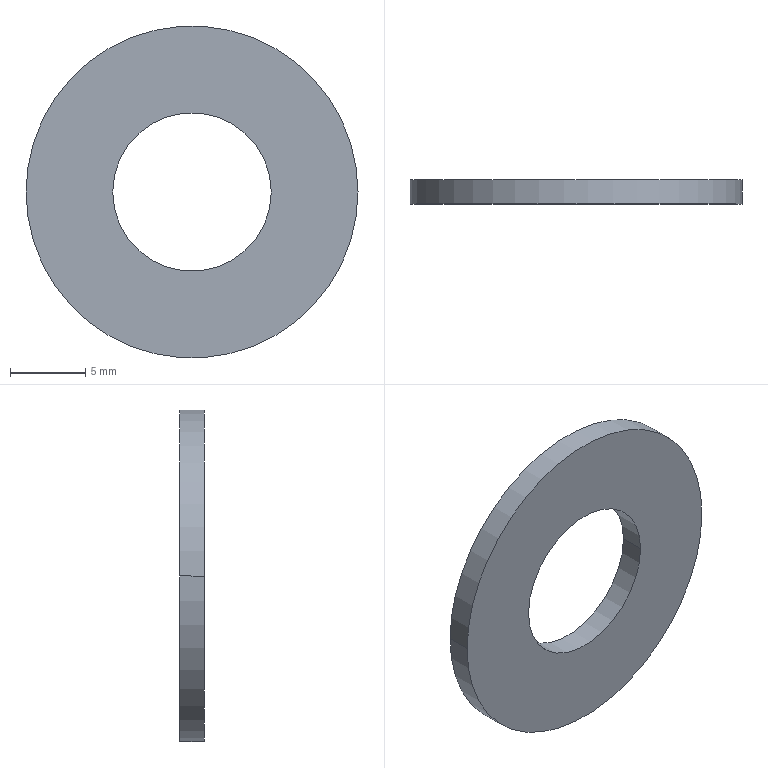Part | STEP file | ZZ21-M10 | 1 solid | 6 faces | box 22 x 1.6 x 22 mm | volume 469.668 mm3 | cylinder 4 | plane 2 | commonest cylinder face diameters 10.5 x2 22 x2
STEP:
#1=CARTESIAN_POINT('',(0.,0.,0.));
#2=DIRECTION('',(0.,0.,1.));
#3=DIRECTION('',(1.,0.,0.));
#4=AXIS2_PLACEMENT_3D('',#1,#2,#3);
#5=CARTESIAN_POINT('',(-5.25,0.,0.));
#6=VERTEX_POINT('',#5);
#7=CARTESIAN_POINT('',(-5.25,1.6,0.));
#8=VERTEX_POINT('',#7);
#9=CARTESIAN_POINT('',(-5.25,0.,0.));
#10=DIRECTION('',(0.,1.,0.));
#11=VECTOR('',#10,1.);
#12=LINE('',#9,#11);
#13=CARTESIAN_POINT('',(0.,0.,0.));
#14=DIRECTION('',(0.,1.,0.));
#15=DIRECTION('',(-1.,0.,0.));
#16=AXIS2_PLACEMENT_3D('',#13,#14,#15);
#17=CYLINDRICAL_SURFACE('',#16,5.25);
#18=CARTESIAN_POINT('',(6.283,0.));
#19=DIRECTION('',(0.,1.));
#20=VECTOR('',#19,1.);
#21=LINE('',#18,#20);
#22=(GEOMETRIC_REPRESENTATION_CONTEXT(2)PARAMETRIC_REPRESENTATION_CONTEXT()REPRESENTATION_CONTEXT('',''));
#23=DEFINITIONAL_REPRESENTATION('',(#21),#22);
#24=PCURVE('',#17,#23);
#25=CARTESIAN_POINT('',(0.,0.,0.));
#26=DIRECTION('',(0.,1.,0.));
#27=DIRECTION('',(-1.,0.,0.));
#28=AXIS2_PLACEMENT_3D('',#25,#26,#27);
#29=CYLINDRICAL_SURFACE('',#28,5.25);
#30=CARTESIAN_POINT('',(0.,0.));
#31=DIRECTION('',(0.,1.));
#32=VECTOR('',#31,1.);
#33=LINE('',#30,#32);
#34=(GEOMETRIC_REPRESENTATION_CONTEXT(2)PARAMETRIC_REPRESENTATION_CONTEXT()REPRESENTATION_CONTEXT('',''));
#35=DEFINITIONAL_REPRESENTATION('',(#33),#34);
#36=PCURVE('',#29,#35);
#37=SURFACE_CURVE('',#12,(#24,#36),.PCURVE_S1.);
#38=EDGE_CURVE('',#6,#8,#37,.T.);
#39=ORIENTED_EDGE('',*,*,#38,.T.);
#40=CARTESIAN_POINT('',(5.25,1.6,0.));
#41=VERTEX_POINT('',#40);
#42=CARTESIAN_POINT('',(0.,1.6,0.));
#43=DIRECTION('',(0.,-1.,0.));
#44=DIRECTION('',(1.,0.,0.));
#45=AXIS2_PLACEMENT_3D('',#42,#43,#44);
#46=CIRCLE('',#45,5.25);
#47=CARTESIAN_POINT('',(9.425,1.6));
#48=DIRECTION('',(-1.,0.));
#49=VECTOR('',#48,1.);
#50=LINE('',#47,#49);
#51=(GEOMETRIC_REPRESENTATION_CONTEXT(2)PARAMETRIC_REPRESENTATION_CONTEXT()REPRESENTATION_CONTEXT('',''));
#52=DEFINITIONAL_REPRESENTATION('',(#50),#51);
#53=PCURVE('',#17,#52);
#54=CARTESIAN_POINT('',(0.,1.6,0.));
#55=DIRECTION('',(0.,1.,0.));
#56=DIRECTION('',(-1.,0.,0.));
#57=AXIS2_PLACEMENT_3D('',#54,#55,#56);
#58=PLANE('',#57);
#59=CARTESIAN_POINT('',(-5.25,0.));
#60=CARTESIAN_POINT('',(-5.25,9.093));
#61=CARTESIAN_POINT('',(2.625,4.547));
#62=CARTESIAN_POINT('',(10.5,0.));
#63=CARTESIAN_POINT('',(2.625,-4.547));
#64=CARTESIAN_POINT('',(-5.25,-9.093));
#65=CARTESIAN_POINT('',(-5.25,0.));
#66=(BOUNDED_CURVE()B_SPLINE_CURVE(2,(#59,#60,#61,#62,#63,#64,#65),.UNSPECIFIED.,.T.,.F.)B_SPLINE_CURVE_WITH_KNOTS((1,2,2,2,2,1),(-2.094,0.,2.094,4.189,6.283,8.378),.UNSPECIFIED.)CURVE()GEOMETRIC_REPRESENTATION_ITEM()RATIONAL_B_SPLINE_CURVE((1.,0.5,1.,0.5,1.,0.5,1.))REPRESENTATION_ITEM(''));
#67=(GEOMETRIC_REPRESENTATION_CONTEXT(2)PARAMETRIC_REPRESENTATION_CONTEXT()REPRESENTATION_CONTEXT('',''));
#68=DEFINITIONAL_REPRESENTATION('',(#66),#67);
#69=PCURVE('',#58,#68);
#70=SURFACE_CURVE('',#46,(#53,#69),.PCURVE_S1.);
#71=EDGE_CURVE('',#8,#41,#70,.T.);
#72=ORIENTED_EDGE('',*,*,#71,.T.);
#73=CARTESIAN_POINT('',(5.25,0.,0.));
#74=VERTEX_POINT('',#73);
#75=CARTESIAN_POINT('',(5.25,0.,0.));
#76=DIRECTION('',(0.,1.,0.));
#77=VECTOR('',#76,1.);
#78=LINE('',#75,#77);
#79=CARTESIAN_POINT('',(3.142,0.));
#80=DIRECTION('',(0.,1.));
#81=VECTOR('',#80,1.);
#82=LINE('',#79,#81);
#83=(GEOMETRIC_REPRESENTATION_CONTEXT(2)PARAMETRIC_REPRESENTATION_CONTEXT()REPRESENTATION_CONTEXT('',''));
#84=DEFINITIONAL_REPRESENTATION('',(#82),#83);
#85=PCURVE('',#17,#84);
#86=CARTESIAN_POINT('',(3.142,0.));
#87=DIRECTION('',(0.,1.));
#88=VECTOR('',#87,1.);
#89=LINE('',#86,#88);
#90=(GEOMETRIC_REPRESENTATION_CONTEXT(2)PARAMETRIC_REPRESENTATION_CONTEXT()REPRESENTATION_CONTEXT('',''));
#91=DEFINITIONAL_REPRESENTATION('',(#89),#90);
#92=PCURVE('',#29,#91);
#93=SURFACE_CURVE('',#78,(#85,#92),.PCURVE_S1.);
#94=EDGE_CURVE('',#74,#41,#93,.T.);
#95=ORIENTED_EDGE('',*,*,#94,.F.);
#96=CARTESIAN_POINT('',(0.,0.,0.));
#97=DIRECTION('',(0.,1.,0.));
#98=DIRECTION('',(-1.,0.,0.));
#99=AXIS2_PLACEMENT_3D('',#96,#97,#98);
#100=CIRCLE('',#99,5.25);
#101=CARTESIAN_POINT('',(0.,0.));
#102=DIRECTION('',(1.,0.));
#103=VECTOR('',#102,1.);
#104=LINE('',#101,#103);
#105=(GEOMETRIC_REPRESENTATION_CONTEXT(2)PARAMETRIC_REPRESENTATION_CONTEXT()REPRESENTATION_CONTEXT('',''));
#106=DEFINITIONAL_REPRESENTATION('',(#104),#105);
#107=PCURVE('',#17,#106);
#108=CARTESIAN_POINT('',(0.,0.,0.));
#109=DIRECTION('',(0.,-1.,0.));
#110=DIRECTION('',(1.,0.,0.));
#111=AXIS2_PLACEMENT_3D('',#108,#109,#110);
#112=PLANE('',#111);
#113=CARTESIAN_POINT('',(-5.25,0.));
#114=CARTESIAN_POINT('',(-5.25,9.093));
#115=CARTESIAN_POINT('',(2.625,4.547));
#116=CARTESIAN_POINT('',(10.5,0.));
#117=CARTESIAN_POINT('',(2.625,-4.547));
#118=CARTESIAN_POINT('',(-5.25,-9.093));
#119=CARTESIAN_POINT('',(-5.25,0.));
#120=(BOUNDED_CURVE()B_SPLINE_CURVE(2,(#113,#114,#115,#116,#117,#118,#119),.UNSPECIFIED.,.T.,.F.)B_SPLINE_CURVE_WITH_KNOTS((1,2,2,2,2,1),(-2.094,0.,2.094,4.189,6.283,8.378),.UNSPECIFIED.)CURVE()GEOMETRIC_REPRESENTATION_ITEM()RATIONAL_B_SPLINE_CURVE((1.,0.5,1.,0.5,1.,0.5,1.))REPRESENTATION_ITEM(''));
#121=(GEOMETRIC_REPRESENTATION_CONTEXT(2)PARAMETRIC_REPRESENTATION_CONTEXT()REPRESENTATION_CONTEXT('',''));
#122=DEFINITIONAL_REPRESENTATION('',(#120),#121);
#123=PCURVE('',#112,#122);
#124=SURFACE_CURVE('',#100,(#107,#123),.PCURVE_S1.);
#125=EDGE_CURVE('',#74,#6,#124,.T.);
#126=ORIENTED_EDGE('',*,*,#125,.T.);
#127=EDGE_LOOP('',(#39,#72,#95,#126));
#128=FACE_BOUND('',#127,.F.);
#129=ADVANCED_FACE('',(#128),#17,.F.);
#130=CARTESIAN_POINT('',(-11.,0.,0.));
#131=VERTEX_POINT('',#130);
#132=CARTESIAN_POINT('',(11.,0.,0.));
#133=VERTEX_POINT('',#132);
#134=CARTESIAN_POINT('',(0.,0.,0.));
#135=DIRECTION('',(0.,1.,0.));
#136=DIRECTION('',(-1.,0.,0.));
#137=AXIS2_PLACEMENT_3D('',#134,#135,#136);
#138=CIRCLE('',#137,11.);
#139=CARTESIAN_POINT('',(0.,0.,0.));
#140=DIRECTION('',(0.,1.,0.));
#141=DIRECTION('',(-1.,0.,0.));
#142=AXIS2_PLACEMENT_3D('',#139,#140,#141);
#143=CYLINDRICAL_SURFACE('',#142,11.);
#144=CARTESIAN_POINT('',(0.,0.));
#145=DIRECTION('',(1.,0.));
#146=VECTOR('',#145,1.);
#147=LINE('',#144,#146);
#148=(GEOMETRIC_REPRESENTATION_CONTEXT(2)PARAMETRIC_REPRESENTATION_CONTEXT()REPRESENTATION_CONTEXT('',''));
#149=DEFINITIONAL_REPRESENTATION('',(#147),#148);
#150=PCURVE('',#143,#149);
#151=CARTESIAN_POINT('',(-11.,0.));
#152=CARTESIAN_POINT('',(-11.,19.053));
#153=CARTESIAN_POINT('',(5.5,9.526));
#154=CARTESIAN_POINT('',(22.,0.));
#155=CARTESIAN_POINT('',(5.5,-9.526));
#156=CARTESIAN_POINT('',(-11.,-19.053));
#157=CARTESIAN_POINT('',(-11.,0.));
#158=(BOUNDED_CURVE()B_SPLINE_CURVE(2,(#151,#152,#153,#154,#155,#156,#157),.UNSPECIFIED.,.T.,.F.)B_SPLINE_CURVE_WITH_KNOTS((1,2,2,2,2,1),(-2.094,0.,2.094,4.189,6.283,8.378),.UNSPECIFIED.)CURVE()GEOMETRIC_REPRESENTATION_ITEM()RATIONAL_B_SPLINE_CURVE((1.,0.5,1.,0.5,1.,0.5,1.))REPRESENTATION_ITEM(''));
#159=(GEOMETRIC_REPRESENTATION_CONTEXT(2)PARAMETRIC_REPRESENTATION_CONTEXT()REPRESENTATION_CONTEXT('',''));
#160=DEFINITIONAL_REPRESENTATION('',(#158),#159);
#161=PCURVE('',#112,#160);
#162=SURFACE_CURVE('',#138,(#150,#161),.PCURVE_S1.);
#163=EDGE_CURVE('',#131,#133,#162,.T.);
#164=ORIENTED_EDGE('',*,*,#163,.T.);
#165=CARTESIAN_POINT('',(11.,1.6,0.));
#166=VERTEX_POINT('',#165);
#167=CARTESIAN_POINT('',(11.,0.,0.));
#168=DIRECTION('',(0.,1.,0.));
#169=VECTOR('',#168,1.);
#170=LINE('',#167,#169);
#171=CARTESIAN_POINT('',(3.142,0.));
#172=DIRECTION('',(0.,1.));
#173=VECTOR('',#172,1.);
#174=LINE('',#171,#173);
#175=(GEOMETRIC_REPRESENTATION_CONTEXT(2)PARAMETRIC_REPRESENTATION_CONTEXT()REPRESENTATION_CONTEXT('',''));
#176=DEFINITIONAL_REPRESENTATION('',(#174),#175);
#177=PCURVE('',#143,#176);
#178=CARTESIAN_POINT('',(0.,0.,0.));
#179=DIRECTION('',(0.,1.,0.));
#180=DIRECTION('',(-1.,0.,0.));
#181=AXIS2_PLACEMENT_3D('',#178,#179,#180);
#182=CYLINDRICAL_SURFACE('',#181,11.);
#183=CARTESIAN_POINT('',(3.142,0.));
#184=DIRECTION('',(0.,1.));
#185=VECTOR('',#184,1.);
#186=LINE('',#183,#185);
#187=(GEOMETRIC_REPRESENTATION_CONTEXT(2)PARAMETRIC_REPRESENTATION_CONTEXT()REPRESENTATION_CONTEXT('',''));
#188=DEFINITIONAL_REPRESENTATION('',(#186),#187);
#189=PCURVE('',#182,#188);
#190=SURFACE_CURVE('',#170,(#177,#189),.PCURVE_S1.);
#191=EDGE_CURVE('',#133,#166,#190,.T.);
#192=ORIENTED_EDGE('',*,*,#191,.T.);
#193=CARTESIAN_POINT('',(-11.,1.6,0.));
#194=VERTEX_POINT('',#193);
#195=CARTESIAN_POINT('',(0.,1.6,0.));
#196=DIRECTION('',(0.,-1.,0.));
#197=DIRECTION('',(1.,0.,0.));
#198=AXIS2_PLACEMENT_3D('',#195,#196,#197);
#199=CIRCLE('',#198,11.);
#200=CARTESIAN_POINT('',(3.142,1.6));
#201=DIRECTION('',(-1.,0.));
#202=VECTOR('',#201,1.);
#203=LINE('',#200,#202);
#204=(GEOMETRIC_REPRESENTATION_CONTEXT(2)PARAMETRIC_REPRESENTATION_CONTEXT()REPRESENTATION_CONTEXT('',''));
#205=DEFINITIONAL_REPRESENTATION('',(#203),#204);
#206=PCURVE('',#143,#205);
#207=CARTESIAN_POINT('',(-11.,0.));
#208=CARTESIAN_POINT('',(-11.,19.053));
#209=CARTESIAN_POINT('',(5.5,9.526));
#210=CARTESIAN_POINT('',(22.,0.));
#211=CARTESIAN_POINT('',(5.5,-9.526));
#212=CARTESIAN_POINT('',(-11.,-19.053));
#213=CARTESIAN_POINT('',(-11.,0.));
#214=(BOUNDED_CURVE()B_SPLINE_CURVE(2,(#207,#208,#209,#210,#211,#212,#213),.UNSPECIFIED.,.T.,.F.)B_SPLINE_CURVE_WITH_KNOTS((1,2,2,2,2,1),(-2.094,0.,2.094,4.189,6.283,8.378),.UNSPECIFIED.)CURVE()GEOMETRIC_REPRESENTATION_ITEM()RATIONAL_B_SPLINE_CURVE((1.,0.5,1.,0.5,1.,0.5,1.))REPRESENTATION_ITEM(''));
#215=(GEOMETRIC_REPRESENTATION_CONTEXT(2)PARAMETRIC_REPRESENTATION_CONTEXT()REPRESENTATION_CONTEXT('',''));
#216=DEFINITIONAL_REPRESENTATION('',(#214),#215);
#217=PCURVE('',#58,#216);
#218=SURFACE_CURVE('',#199,(#206,#217),.PCURVE_S1.);
#219=EDGE_CURVE('',#166,#194,#218,.T.);
#220=ORIENTED_EDGE('',*,*,#219,.T.);
#221=CARTESIAN_POINT('',(-11.,0.,0.));
#222=DIRECTION('',(0.,1.,0.));
#223=VECTOR('',#222,1.);
#224=LINE('',#221,#223);
#225=CARTESIAN_POINT('',(0.,0.));
#226=DIRECTION('',(0.,1.));
#227=VECTOR('',#226,1.);
#228=LINE('',#225,#227);
#229=(GEOMETRIC_REPRESENTATION_CONTEXT(2)PARAMETRIC_REPRESENTATION_CONTEXT()REPRESENTATION_CONTEXT('',''));
#230=DEFINITIONAL_REPRESENTATION('',(#228),#229);
#231=PCURVE('',#143,#230);
#232=CARTESIAN_POINT('',(6.283,0.));
#233=DIRECTION('',(0.,1.));
#234=VECTOR('',#233,1.);
#235=LINE('',#232,#234);
#236=(GEOMETRIC_REPRESENTATION_CONTEXT(2)PARAMETRIC_REPRESENTATION_CONTEXT()REPRESENTATION_CONTEXT('',''));
#237=DEFINITIONAL_REPRESENTATION('',(#235),#236);
#238=PCURVE('',#182,#237);
#239=SURFACE_CURVE('',#224,(#231,#238),.PCURVE_S1.);
#240=EDGE_CURVE('',#131,#194,#239,.T.);
#241=ORIENTED_EDGE('',*,*,#240,.F.);
#242=EDGE_LOOP('',(#164,#192,#220,#241));
#243=FACE_BOUND('',#242,.T.);
#244=ADVANCED_FACE('',(#243),#143,.T.);
#245=ORIENTED_EDGE('',*,*,#71,.T.);
#246=CARTESIAN_POINT('',(0.,1.6,0.));
#247=DIRECTION('',(0.,-1.,0.));
#248=DIRECTION('',(1.,0.,0.));
#249=AXIS2_PLACEMENT_3D('',#246,#247,#248);
#250=CIRCLE('',#249,5.25);
#251=CARTESIAN_POINT('',(-5.25,0.));
#252=CARTESIAN_POINT('',(-5.25,9.093));
#253=CARTESIAN_POINT('',(2.625,4.547));
#254=CARTESIAN_POINT('',(10.5,0.));
#255=CARTESIAN_POINT('',(2.625,-4.547));
#256=CARTESIAN_POINT('',(-5.25,-9.093));
#257=CARTESIAN_POINT('',(-5.25,0.));
#258=(BOUNDED_CURVE()B_SPLINE_CURVE(2,(#251,#252,#253,#254,#255,#256,#257),.UNSPECIFIED.,.T.,.F.)B_SPLINE_CURVE_WITH_KNOTS((1,2,2,2,2,1),(-2.094,0.,2.094,4.189,6.283,8.378),.UNSPECIFIED.)CURVE()GEOMETRIC_REPRESENTATION_ITEM()RATIONAL_B_SPLINE_CURVE((1.,0.5,1.,0.5,1.,0.5,1.))REPRESENTATION_ITEM(''));
#259=(GEOMETRIC_REPRESENTATION_CONTEXT(2)PARAMETRIC_REPRESENTATION_CONTEXT()REPRESENTATION_CONTEXT('',''));
#260=DEFINITIONAL_REPRESENTATION('',(#258),#259);
#261=PCURVE('',#58,#260);
#262=CARTESIAN_POINT('',(3.142,1.6));
#263=DIRECTION('',(-1.,0.));
#264=VECTOR('',#263,1.);
#265=LINE('',#262,#264);
#266=(GEOMETRIC_REPRESENTATION_CONTEXT(2)PARAMETRIC_REPRESENTATION_CONTEXT()REPRESENTATION_CONTEXT('',''));
#267=DEFINITIONAL_REPRESENTATION('',(#265),#266);
#268=PCURVE('',#29,#267);
#269=SURFACE_CURVE('',#250,(#261,#268),.PCURVE_S1.);
#270=EDGE_CURVE('',#41,#8,#269,.T.);
#271=ORIENTED_EDGE('',*,*,#270,.T.);
#272=EDGE_LOOP('',(#245,#271));
#273=FACE_BOUND('',#272,.T.);
#274=CARTESIAN_POINT('',(0.,1.6,0.));
#275=DIRECTION('',(0.,-1.,0.));
#276=DIRECTION('',(1.,0.,0.));
#277=AXIS2_PLACEMENT_3D('',#274,#275,#276);
#278=CIRCLE('',#277,11.);
#279=CARTESIAN_POINT('',(-11.,0.));
#280=CARTESIAN_POINT('',(-11.,19.053));
#281=CARTESIAN_POINT('',(5.5,9.526));
#282=CARTESIAN_POINT('',(22.,0.));
#283=CARTESIAN_POINT('',(5.5,-9.526));
#284=CARTESIAN_POINT('',(-11.,-19.053));
#285=CARTESIAN_POINT('',(-11.,0.));
#286=(BOUNDED_CURVE()B_SPLINE_CURVE(2,(#279,#280,#281,#282,#283,#284,#285),.UNSPECIFIED.,.T.,.F.)B_SPLINE_CURVE_WITH_KNOTS((1,2,2,2,2,1),(-2.094,0.,2.094,4.189,6.283,8.378),.UNSPECIFIED.)CURVE()GEOMETRIC_REPRESENTATION_ITEM()RATIONAL_B_SPLINE_CURVE((1.,0.5,1.,0.5,1.,0.5,1.))REPRESENTATION_ITEM(''));
#287=(GEOMETRIC_REPRESENTATION_CONTEXT(2)PARAMETRIC_REPRESENTATION_CONTEXT()REPRESENTATION_CONTEXT('',''));
#288=DEFINITIONAL_REPRESENTATION('',(#286),#287);
#289=PCURVE('',#58,#288);
#290=CARTESIAN_POINT('',(9.425,1.6));
#291=DIRECTION('',(-1.,0.));
#292=VECTOR('',#291,1.);
#293=LINE('',#290,#292);
#294=(GEOMETRIC_REPRESENTATION_CONTEXT(2)PARAMETRIC_REPRESENTATION_CONTEXT()REPRESENTATION_CONTEXT('',''));
#295=DEFINITIONAL_REPRESENTATION('',(#293),#294);
#296=PCURVE('',#182,#295);
#297=SURFACE_CURVE('',#278,(#289,#296),.PCURVE_S1.);
#298=EDGE_CURVE('',#194,#166,#297,.T.);
#299=ORIENTED_EDGE('',*,*,#298,.F.);
#300=ORIENTED_EDGE('',*,*,#219,.F.);
#301=EDGE_LOOP('',(#299,#300));
#302=FACE_BOUND('',#301,.T.);
#303=ADVANCED_FACE('',(#273,#302),#58,.T.);
#304=CARTESIAN_POINT('',(0.,0.,0.));
#305=DIRECTION('',(0.,1.,0.));
#306=DIRECTION('',(-1.,0.,0.));
#307=AXIS2_PLACEMENT_3D('',#304,#305,#306);
#308=CIRCLE('',#307,5.25);
#309=CARTESIAN_POINT('',(-5.25,0.));
#310=CARTESIAN_POINT('',(-5.25,9.093));
#311=CARTESIAN_POINT('',(2.625,4.547));
#312=CARTESIAN_POINT('',(10.5,0.));
#313=CARTESIAN_POINT('',(2.625,-4.547));
#314=CARTESIAN_POINT('',(-5.25,-9.093));
#315=CARTESIAN_POINT('',(-5.25,0.));
#316=(BOUNDED_CURVE()B_SPLINE_CURVE(2,(#309,#310,#311,#312,#313,#314,#315),.UNSPECIFIED.,.T.,.F.)B_SPLINE_CURVE_WITH_KNOTS((1,2,2,2,2,1),(-2.094,0.,2.094,4.189,6.283,8.378),.UNSPECIFIED.)CURVE()GEOMETRIC_REPRESENTATION_ITEM()RATIONAL_B_SPLINE_CURVE((1.,0.5,1.,0.5,1.,0.5,1.))REPRESENTATION_ITEM(''));
#317=(GEOMETRIC_REPRESENTATION_CONTEXT(2)PARAMETRIC_REPRESENTATION_CONTEXT()REPRESENTATION_CONTEXT('',''));
#318=DEFINITIONAL_REPRESENTATION('',(#316),#317);
#319=PCURVE('',#112,#318);
#320=CARTESIAN_POINT('',(0.,0.));
#321=DIRECTION('',(1.,0.));
#322=VECTOR('',#321,1.);
#323=LINE('',#320,#322);
#324=(GEOMETRIC_REPRESENTATION_CONTEXT(2)PARAMETRIC_REPRESENTATION_CONTEXT()REPRESENTATION_CONTEXT('',''));
#325=DEFINITIONAL_REPRESENTATION('',(#323),#324);
#326=PCURVE('',#29,#325);
#327=SURFACE_CURVE('',#308,(#319,#326),.PCURVE_S1.);
#328=EDGE_CURVE('',#6,#74,#327,.T.);
#329=ORIENTED_EDGE('',*,*,#328,.T.);
#330=ORIENTED_EDGE('',*,*,#125,.T.);
#331=EDGE_LOOP('',(#329,#330));
#332=FACE_BOUND('',#331,.T.);
#333=ORIENTED_EDGE('',*,*,#163,.F.);
#334=CARTESIAN_POINT('',(0.,0.,0.));
#335=DIRECTION('',(0.,1.,0.));
#336=DIRECTION('',(-1.,0.,0.));
#337=AXIS2_PLACEMENT_3D('',#334,#335,#336);
#338=CIRCLE('',#337,11.);
#339=CARTESIAN_POINT('',(-11.,0.));
#340=CARTESIAN_POINT('',(-11.,19.053));
#341=CARTESIAN_POINT('',(5.5,9.526));
#342=CARTESIAN_POINT('',(22.,0.));
#343=CARTESIAN_POINT('',(5.5,-9.526));
#344=CARTESIAN_POINT('',(-11.,-19.053));
#345=CARTESIAN_POINT('',(-11.,0.));
#346=(BOUNDED_CURVE()B_SPLINE_CURVE(2,(#339,#340,#341,#342,#343,#344,#345),.UNSPECIFIED.,.T.,.F.)B_SPLINE_CURVE_WITH_KNOTS((1,2,2,2,2,1),(-2.094,0.,2.094,4.189,6.283,8.378),.UNSPECIFIED.)CURVE()GEOMETRIC_REPRESENTATION_ITEM()RATIONAL_B_SPLINE_CURVE((1.,0.5,1.,0.5,1.,0.5,1.))REPRESENTATION_ITEM(''));
#347=(GEOMETRIC_REPRESENTATION_CONTEXT(2)PARAMETRIC_REPRESENTATION_CONTEXT()REPRESENTATION_CONTEXT('',''));
#348=DEFINITIONAL_REPRESENTATION('',(#346),#347);
#349=PCURVE('',#112,#348);
#350=CARTESIAN_POINT('',(0.,0.));
#351=DIRECTION('',(1.,0.));
#352=VECTOR('',#351,1.);
#353=LINE('',#350,#352);
#354=(GEOMETRIC_REPRESENTATION_CONTEXT(2)PARAMETRIC_REPRESENTATION_CONTEXT()REPRESENTATION_CONTEXT('',''));
#355=DEFINITIONAL_REPRESENTATION('',(#353),#354);
#356=PCURVE('',#182,#355);
#357=SURFACE_CURVE('',#338,(#349,#356),.PCURVE_S1.);
#358=EDGE_CURVE('',#133,#131,#357,.T.);
#359=ORIENTED_EDGE('',*,*,#358,.F.);
#360=EDGE_LOOP('',(#333,#359));
#361=FACE_BOUND('',#360,.T.);
#362=ADVANCED_FACE('',(#332,#361),#112,.T.);
#363=ORIENTED_EDGE('',*,*,#191,.F.);
#364=ORIENTED_EDGE('',*,*,#358,.T.);
#365=ORIENTED_EDGE('',*,*,#240,.T.);
#366=ORIENTED_EDGE('',*,*,#298,.T.);
#367=EDGE_LOOP('',(#363,#364,#365,#366));
#368=FACE_BOUND('',#367,.T.);
#369=ADVANCED_FACE('',(#368),#182,.T.);
#370=ORIENTED_EDGE('',*,*,#270,.T.);
#371=ORIENTED_EDGE('',*,*,#38,.F.);
#372=ORIENTED_EDGE('',*,*,#328,.T.);
#373=ORIENTED_EDGE('',*,*,#94,.T.);
#374=EDGE_LOOP('',(#370,#371,#372,#373));
#375=FACE_BOUND('',#374,.F.);
#376=ADVANCED_FACE('',(#375),#29,.F.);
#377=CLOSED_SHELL('',(#129,#244,#303,#362,#369,#376));
#378=MANIFOLD_SOLID_BREP('',#377);
#379=(LENGTH_UNIT()NAMED_UNIT(*)SI_UNIT(.MILLI.,.METRE.));
#380=UNCERTAINTY_MEASURE_WITH_UNIT(LENGTH_MEASURE(0.0000001),#379,'','');
#381=(NAMED_UNIT(*)PLANE_ANGLE_UNIT()SI_UNIT($,.RADIAN.));
#382=(NAMED_UNIT(*)SI_UNIT($,.STERADIAN.)SOLID_ANGLE_UNIT());
#383=(GEOMETRIC_REPRESENTATION_CONTEXT(3)GLOBAL_UNCERTAINTY_ASSIGNED_CONTEXT((#380))GLOBAL_UNIT_ASSIGNED_CONTEXT((#379,#381,#382))REPRESENTATION_CONTEXT('',''));
#384=ADVANCED_BREP_SHAPE_REPRESENTATION('',(#4,#378),#383);